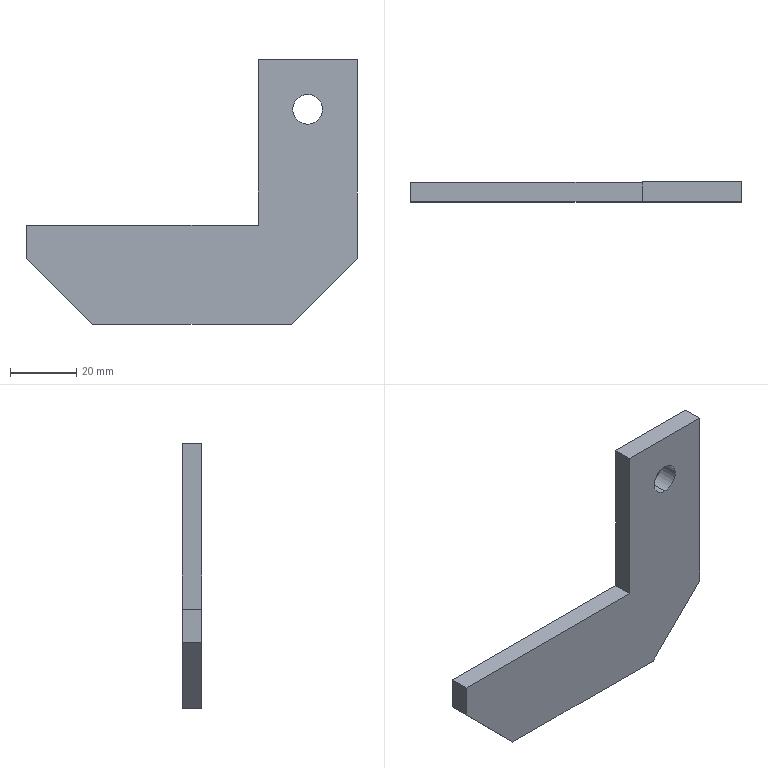Part | SolidWorks | features Chamfer 2, Extrusion 1, ICE 1 | 1 solid | 12 faces | box 100 x 6 x 80 mm | volume 24218 mm3 | plane 10 | cylinder 2 | commonest cylinder face diameters 9 x2
STEP:
#1=CARTESIAN_POINT('',(66.923,0.,-1.423));
#2=VERTEX_POINT('',#1);
#3=CARTESIAN_POINT('',(66.923,0.,7.577));
#4=VERTEX_POINT('',#3);
#5=CARTESIAN_POINT('',(66.923,0.,3.077));
#6=DIRECTION('',(0.,1.,0.));
#7=DIRECTION('',(0.,0.,1.));
#8=AXIS2_PLACEMENT_3D('',#5,#6,#7);
#9=CIRCLE('',#8,4.5);
#10=EDGE_CURVE('',#2,#4,#9,.T.);
#11=ORIENTED_EDGE('',*,*,#10,.F.);
#12=CARTESIAN_POINT('',(66.923,6.,-1.423));
#13=VERTEX_POINT('',#12);
#14=CARTESIAN_POINT('',(66.923,0.,-1.423));
#15=DIRECTION('',(0.,1.,0.));
#16=VECTOR('',#15,1000.);
#17=LINE('',#14,#16);
#18=EDGE_CURVE('',#2,#13,#17,.T.);
#19=ORIENTED_EDGE('',*,*,#18,.T.);
#20=CARTESIAN_POINT('',(66.923,6.,7.577));
#21=VERTEX_POINT('',#20);
#22=CARTESIAN_POINT('',(66.923,6.,3.077));
#23=DIRECTION('',(0.,1.,0.));
#24=DIRECTION('',(0.,0.,1.));
#25=AXIS2_PLACEMENT_3D('',#22,#23,#24);
#26=CIRCLE('',#25,4.5);
#27=EDGE_CURVE('',#13,#21,#26,.T.);
#28=ORIENTED_EDGE('',*,*,#27,.T.);
#29=CARTESIAN_POINT('',(66.923,0.,7.577));
#30=DIRECTION('',(0.,1.,0.));
#31=VECTOR('',#30,1000.);
#32=LINE('',#29,#31);
#33=EDGE_CURVE('',#4,#21,#32,.T.);
#34=ORIENTED_EDGE('',*,*,#33,.F.);
#35=EDGE_LOOP('',(#11,#19,#28,#34));
#36=FACE_OUTER_BOUND('',#35,.T.);
#37=CARTESIAN_POINT('',(66.923,0.,3.077));
#38=DIRECTION('',(0.,1.,0.));
#39=DIRECTION('',(0.,0.,1.));
#40=AXIS2_PLACEMENT_3D('',#37,#38,#39);
#41=CYLINDRICAL_SURFACE('',#40,4.5);
#42=ADVANCED_FACE('',(#36),#41,.F.);
#43=CARTESIAN_POINT('',(-18.077,6.,-41.923));
#44=VERTEX_POINT('',#43);
#45=CARTESIAN_POINT('',(-18.077,6.,-31.923));
#46=VERTEX_POINT('',#45);
#47=CARTESIAN_POINT('',(-18.077,6.,-31.923));
#48=DIRECTION('',(0.,0.,1.));
#49=VECTOR('',#48,1000.);
#50=LINE('',#47,#49);
#51=EDGE_CURVE('',#44,#46,#50,.T.);
#52=ORIENTED_EDGE('',*,*,#51,.F.);
#53=CARTESIAN_POINT('',(-18.077,0.,-41.923));
#54=VERTEX_POINT('',#53);
#55=CARTESIAN_POINT('',(-18.077,6.,-41.923));
#56=DIRECTION('',(0.,-1.,0.));
#57=VECTOR('',#56,1000.);
#58=LINE('',#55,#57);
#59=EDGE_CURVE('',#44,#54,#58,.T.);
#60=ORIENTED_EDGE('',*,*,#59,.T.);
#61=CARTESIAN_POINT('',(-18.077,0.,-31.923));
#62=VERTEX_POINT('',#61);
#63=CARTESIAN_POINT('',(-18.077,0.,-31.923));
#64=DIRECTION('',(0.,0.,1.));
#65=VECTOR('',#64,1000.);
#66=LINE('',#63,#65);
#67=EDGE_CURVE('',#54,#62,#66,.T.);
#68=ORIENTED_EDGE('',*,*,#67,.T.);
#69=CARTESIAN_POINT('',(-18.077,6.,-31.923));
#70=DIRECTION('',(0.,-1.,0.));
#71=VECTOR('',#70,1000.);
#72=LINE('',#69,#71);
#73=EDGE_CURVE('',#46,#62,#72,.T.);
#74=ORIENTED_EDGE('',*,*,#73,.F.);
#75=EDGE_LOOP('',(#52,#60,#68,#74));
#76=FACE_OUTER_BOUND('',#75,.T.);
#77=CARTESIAN_POINT('',(-18.077,6.,-31.923));
#78=DIRECTION('',(1.,0.,0.));
#79=DIRECTION('',(0.,0.,-1.));
#80=AXIS2_PLACEMENT_3D('',#77,#78,#79);
#81=PLANE('',#80);
#82=ADVANCED_FACE('',(#76),#81,.F.);
#83=CARTESIAN_POINT('',(51.923,0.,-31.923));
#84=VERTEX_POINT('',#83);
#85=CARTESIAN_POINT('',(51.923,0.,-31.923));
#86=DIRECTION('',(1.,0.,0.));
#87=VECTOR('',#86,1000.);
#88=LINE('',#85,#87);
#89=EDGE_CURVE('',#62,#84,#88,.T.);
#90=ORIENTED_EDGE('',*,*,#89,.T.);
#91=CARTESIAN_POINT('',(51.923,6.,-31.923));
#92=VERTEX_POINT('',#91);
#93=CARTESIAN_POINT('',(51.923,6.,-31.923));
#94=DIRECTION('',(0.,-1.,0.));
#95=VECTOR('',#94,1000.);
#96=LINE('',#93,#95);
#97=EDGE_CURVE('',#92,#84,#96,.T.);
#98=ORIENTED_EDGE('',*,*,#97,.F.);
#99=CARTESIAN_POINT('',(51.923,6.,-31.923));
#100=DIRECTION('',(1.,0.,0.));
#101=VECTOR('',#100,1000.);
#102=LINE('',#99,#101);
#103=EDGE_CURVE('',#46,#92,#102,.T.);
#104=ORIENTED_EDGE('',*,*,#103,.F.);
#105=ORIENTED_EDGE('',*,*,#73,.T.);
#106=EDGE_LOOP('',(#90,#98,#104,#105));
#107=FACE_OUTER_BOUND('',#106,.T.);
#108=CARTESIAN_POINT('',(51.923,6.,-31.923));
#109=DIRECTION('',(0.,0.,-1.));
#110=DIRECTION('',(-1.,0.,0.));
#111=AXIS2_PLACEMENT_3D('',#108,#109,#110);
#112=PLANE('',#111);
#113=ADVANCED_FACE('',(#107),#112,.F.);
#114=CARTESIAN_POINT('',(51.923,0.,18.077));
#115=VERTEX_POINT('',#114);
#116=CARTESIAN_POINT('',(51.923,0.,18.077));
#117=DIRECTION('',(0.,0.,1.));
#118=VECTOR('',#117,1000.);
#119=LINE('',#116,#118);
#120=EDGE_CURVE('',#84,#115,#119,.T.);
#121=ORIENTED_EDGE('',*,*,#120,.T.);
#122=CARTESIAN_POINT('',(51.923,6.,18.077));
#123=VERTEX_POINT('',#122);
#124=CARTESIAN_POINT('',(51.923,6.,18.077));
#125=DIRECTION('',(0.,-1.,0.));
#126=VECTOR('',#125,1000.);
#127=LINE('',#124,#126);
#128=EDGE_CURVE('',#123,#115,#127,.T.);
#129=ORIENTED_EDGE('',*,*,#128,.F.);
#130=CARTESIAN_POINT('',(51.923,6.,18.077));
#131=DIRECTION('',(0.,0.,1.));
#132=VECTOR('',#131,1000.);
#133=LINE('',#130,#132);
#134=EDGE_CURVE('',#92,#123,#133,.T.);
#135=ORIENTED_EDGE('',*,*,#134,.F.);
#136=ORIENTED_EDGE('',*,*,#97,.T.);
#137=EDGE_LOOP('',(#121,#129,#135,#136));
#138=FACE_OUTER_BOUND('',#137,.T.);
#139=CARTESIAN_POINT('',(51.923,6.,18.077));
#140=DIRECTION('',(1.,0.,0.));
#141=DIRECTION('',(0.,0.,-1.));
#142=AXIS2_PLACEMENT_3D('',#139,#140,#141);
#143=PLANE('',#142);
#144=ADVANCED_FACE('',(#138),#143,.F.);
#145=CARTESIAN_POINT('',(81.923,0.,18.077));
#146=VERTEX_POINT('',#145);
#147=CARTESIAN_POINT('',(81.923,0.,18.077));
#148=DIRECTION('',(1.,0.,0.));
#149=VECTOR('',#148,1000.);
#150=LINE('',#147,#149);
#151=EDGE_CURVE('',#115,#146,#150,.T.);
#152=ORIENTED_EDGE('',*,*,#151,.T.);
#153=CARTESIAN_POINT('',(81.923,6.,18.077));
#154=VERTEX_POINT('',#153);
#155=CARTESIAN_POINT('',(81.923,6.,18.077));
#156=DIRECTION('',(0.,-1.,0.));
#157=VECTOR('',#156,1000.);
#158=LINE('',#155,#157);
#159=EDGE_CURVE('',#154,#146,#158,.T.);
#160=ORIENTED_EDGE('',*,*,#159,.F.);
#161=CARTESIAN_POINT('',(81.923,6.,18.077));
#162=DIRECTION('',(1.,0.,0.));
#163=VECTOR('',#162,1000.);
#164=LINE('',#161,#163);
#165=EDGE_CURVE('',#123,#154,#164,.T.);
#166=ORIENTED_EDGE('',*,*,#165,.F.);
#167=ORIENTED_EDGE('',*,*,#128,.T.);
#168=EDGE_LOOP('',(#152,#160,#166,#167));
#169=FACE_OUTER_BOUND('',#168,.T.);
#170=CARTESIAN_POINT('',(81.923,6.,18.077));
#171=DIRECTION('',(0.,0.,-1.));
#172=DIRECTION('',(-1.,0.,0.));
#173=AXIS2_PLACEMENT_3D('',#170,#171,#172);
#174=PLANE('',#173);
#175=ADVANCED_FACE('',(#169),#174,.F.);
#176=CARTESIAN_POINT('',(81.923,0.,-41.923));
#177=VERTEX_POINT('',#176);
#178=CARTESIAN_POINT('',(81.923,0.,-61.923));
#179=DIRECTION('',(0.,0.,-1.));
#180=VECTOR('',#179,1000.);
#181=LINE('',#178,#180);
#182=EDGE_CURVE('',#146,#177,#181,.T.);
#183=ORIENTED_EDGE('',*,*,#182,.T.);
#184=CARTESIAN_POINT('',(81.923,6.,-41.923));
#185=VERTEX_POINT('',#184);
#186=CARTESIAN_POINT('',(81.923,6.,-41.923));
#187=DIRECTION('',(0.,1.,0.));
#188=VECTOR('',#187,1000.);
#189=LINE('',#186,#188);
#190=EDGE_CURVE('',#177,#185,#189,.T.);
#191=ORIENTED_EDGE('',*,*,#190,.T.);
#192=CARTESIAN_POINT('',(81.923,6.,-61.923));
#193=DIRECTION('',(0.,0.,-1.));
#194=VECTOR('',#193,1000.);
#195=LINE('',#192,#194);
#196=EDGE_CURVE('',#154,#185,#195,.T.);
#197=ORIENTED_EDGE('',*,*,#196,.F.);
#198=ORIENTED_EDGE('',*,*,#159,.T.);
#199=EDGE_LOOP('',(#183,#191,#197,#198));
#200=FACE_OUTER_BOUND('',#199,.T.);
#201=CARTESIAN_POINT('',(81.923,6.,-61.923));
#202=DIRECTION('',(-1.,0.,0.));
#203=DIRECTION('',(0.,0.,1.));
#204=AXIS2_PLACEMENT_3D('',#201,#202,#203);
#205=PLANE('',#204);
#206=ADVANCED_FACE('',(#200),#205,.F.);
#207=CARTESIAN_POINT('',(61.923,6.,-61.923));
#208=VERTEX_POINT('',#207);
#209=CARTESIAN_POINT('',(1.923,6.,-61.923));
#210=VERTEX_POINT('',#209);
#211=CARTESIAN_POINT('',(-18.077,6.,-61.923));
#212=DIRECTION('',(-1.,0.,0.));
#213=VECTOR('',#212,1000.);
#214=LINE('',#211,#213);
#215=EDGE_CURVE('',#208,#210,#214,.T.);
#216=ORIENTED_EDGE('',*,*,#215,.F.);
#217=CARTESIAN_POINT('',(61.923,0.,-61.923));
#218=VERTEX_POINT('',#217);
#219=CARTESIAN_POINT('',(61.923,6.,-61.923));
#220=DIRECTION('',(0.,-1.,0.));
#221=VECTOR('',#220,1000.);
#222=LINE('',#219,#221);
#223=EDGE_CURVE('',#208,#218,#222,.T.);
#224=ORIENTED_EDGE('',*,*,#223,.T.);
#225=CARTESIAN_POINT('',(1.923,0.,-61.923));
#226=VERTEX_POINT('',#225);
#227=CARTESIAN_POINT('',(-18.077,0.,-61.923));
#228=DIRECTION('',(-1.,0.,0.));
#229=VECTOR('',#228,1000.);
#230=LINE('',#227,#229);
#231=EDGE_CURVE('',#218,#226,#230,.T.);
#232=ORIENTED_EDGE('',*,*,#231,.T.);
#233=CARTESIAN_POINT('',(1.923,6.,-61.923));
#234=DIRECTION('',(0.,1.,0.));
#235=VECTOR('',#234,1000.);
#236=LINE('',#233,#235);
#237=EDGE_CURVE('',#226,#210,#236,.T.);
#238=ORIENTED_EDGE('',*,*,#237,.T.);
#239=EDGE_LOOP('',(#216,#224,#232,#238));
#240=FACE_OUTER_BOUND('',#239,.T.);
#241=CARTESIAN_POINT('',(-18.077,6.,-61.923));
#242=DIRECTION('',(0.,0.,1.));
#243=DIRECTION('',(1.,0.,0.));
#244=AXIS2_PLACEMENT_3D('',#241,#242,#243);
#245=PLANE('',#244);
#246=ADVANCED_FACE('',(#240),#245,.F.);
#247=CARTESIAN_POINT('',(66.923,6.,3.077));
#248=DIRECTION('',(0.,1.,0.));
#249=DIRECTION('',(0.,0.,1.));
#250=AXIS2_PLACEMENT_3D('',#247,#248,#249);
#251=CIRCLE('',#250,4.5);
#252=EDGE_CURVE('',#21,#13,#251,.T.);
#253=ORIENTED_EDGE('',*,*,#252,.F.);
#254=ORIENTED_EDGE('',*,*,#27,.F.);
#255=EDGE_LOOP('',(#253,#254));
#256=FACE_BOUND('',#255,.T.);
#257=ORIENTED_EDGE('',*,*,#196,.T.);
#258=CARTESIAN_POINT('',(61.923,6.,-61.923));
#259=DIRECTION('',(-0.7071,0.,-0.7071));
#260=VECTOR('',#259,1000.);
#261=LINE('',#258,#260);
#262=EDGE_CURVE('',#185,#208,#261,.T.);
#263=ORIENTED_EDGE('',*,*,#262,.T.);
#264=ORIENTED_EDGE('',*,*,#215,.T.);
#265=CARTESIAN_POINT('',(-18.077,6.,-41.923));
#266=DIRECTION('',(-0.7071,0.,0.7071));
#267=VECTOR('',#266,1000.);
#268=LINE('',#265,#267);
#269=EDGE_CURVE('',#210,#44,#268,.T.);
#270=ORIENTED_EDGE('',*,*,#269,.T.);
#271=ORIENTED_EDGE('',*,*,#51,.T.);
#272=ORIENTED_EDGE('',*,*,#103,.T.);
#273=ORIENTED_EDGE('',*,*,#134,.T.);
#274=ORIENTED_EDGE('',*,*,#165,.T.);
#275=EDGE_LOOP('',(#257,#263,#264,#270,#271,#272,#273,#274));
#276=FACE_OUTER_BOUND('',#275,.T.);
#277=CARTESIAN_POINT('',(0.,6.,0.));
#278=DIRECTION('',(0.,-1.,0.));
#279=DIRECTION('',(0.,0.,-1.));
#280=AXIS2_PLACEMENT_3D('',#277,#278,#279);
#281=PLANE('',#280);
#282=ADVANCED_FACE('',(#256,#276),#281,.F.);
#283=CARTESIAN_POINT('',(66.923,0.,3.077));
#284=DIRECTION('',(0.,1.,0.));
#285=DIRECTION('',(0.,0.,1.));
#286=AXIS2_PLACEMENT_3D('',#283,#284,#285);
#287=CIRCLE('',#286,4.5);
#288=EDGE_CURVE('',#4,#2,#287,.T.);
#289=ORIENTED_EDGE('',*,*,#288,.T.);
#290=ORIENTED_EDGE('',*,*,#10,.T.);
#291=EDGE_LOOP('',(#289,#290));
#292=FACE_BOUND('',#291,.T.);
#293=ORIENTED_EDGE('',*,*,#231,.F.);
#294=CARTESIAN_POINT('',(61.923,0.,-61.923));
#295=DIRECTION('',(0.7071,0.,0.7071));
#296=VECTOR('',#295,1000.);
#297=LINE('',#294,#296);
#298=EDGE_CURVE('',#218,#177,#297,.T.);
#299=ORIENTED_EDGE('',*,*,#298,.T.);
#300=ORIENTED_EDGE('',*,*,#182,.F.);
#301=ORIENTED_EDGE('',*,*,#151,.F.);
#302=ORIENTED_EDGE('',*,*,#120,.F.);
#303=ORIENTED_EDGE('',*,*,#89,.F.);
#304=ORIENTED_EDGE('',*,*,#67,.F.);
#305=CARTESIAN_POINT('',(-30.,0.,-30.));
#306=DIRECTION('',(0.7071,0.,-0.7071));
#307=VECTOR('',#306,1000.);
#308=LINE('',#305,#307);
#309=EDGE_CURVE('',#54,#226,#308,.T.);
#310=ORIENTED_EDGE('',*,*,#309,.T.);
#311=EDGE_LOOP('',(#293,#299,#300,#301,#302,#303,#304,#310));
#312=FACE_OUTER_BOUND('',#311,.T.);
#313=CARTESIAN_POINT('',(0.,0.,0.));
#314=DIRECTION('',(0.,-1.,0.));
#315=DIRECTION('',(0.,0.,-1.));
#316=AXIS2_PLACEMENT_3D('',#313,#314,#315);
#317=PLANE('',#316);
#318=ADVANCED_FACE('',(#292,#312),#317,.T.);
#319=ORIENTED_EDGE('',*,*,#18,.F.);
#320=ORIENTED_EDGE('',*,*,#288,.F.);
#321=ORIENTED_EDGE('',*,*,#33,.T.);
#322=ORIENTED_EDGE('',*,*,#252,.T.);
#323=EDGE_LOOP('',(#319,#320,#321,#322));
#324=FACE_OUTER_BOUND('',#323,.T.);
#325=CARTESIAN_POINT('',(66.923,0.,3.077));
#326=DIRECTION('',(0.,1.,0.));
#327=DIRECTION('',(0.,0.,1.));
#328=AXIS2_PLACEMENT_3D('',#325,#326,#327);
#329=CYLINDRICAL_SURFACE('',#328,4.5);
#330=ADVANCED_FACE('',(#324),#329,.F.);
#331=ORIENTED_EDGE('',*,*,#269,.F.);
#332=ORIENTED_EDGE('',*,*,#237,.F.);
#333=ORIENTED_EDGE('',*,*,#309,.F.);
#334=ORIENTED_EDGE('',*,*,#59,.F.);
#335=EDGE_LOOP('',(#331,#332,#333,#334));
#336=FACE_OUTER_BOUND('',#335,.T.);
#337=CARTESIAN_POINT('',(-18.077,6.,-41.923));
#338=DIRECTION('',(0.7071,0.,0.7071));
#339=DIRECTION('',(0.,-1.,0.));
#340=AXIS2_PLACEMENT_3D('',#337,#338,#339);
#341=PLANE('',#340);
#342=ADVANCED_FACE('',(#336),#341,.F.);
#343=ORIENTED_EDGE('',*,*,#262,.F.);
#344=ORIENTED_EDGE('',*,*,#190,.F.);
#345=ORIENTED_EDGE('',*,*,#298,.F.);
#346=ORIENTED_EDGE('',*,*,#223,.F.);
#347=EDGE_LOOP('',(#343,#344,#345,#346));
#348=FACE_OUTER_BOUND('',#347,.T.);
#349=CARTESIAN_POINT('',(61.923,6.,-61.923));
#350=DIRECTION('',(-0.7071,0.,0.7071));
#351=DIRECTION('',(0.,-1.,0.));
#352=AXIS2_PLACEMENT_3D('',#349,#350,#351);
#353=PLANE('',#352);
#354=ADVANCED_FACE('',(#348),#353,.F.);
#355=CLOSED_SHELL('',(#42,#82,#113,#144,#175,#206,#246,#282,#318,#330,#342,#354));
#356=MANIFOLD_SOLID_BREP('',#355);
#357=CARTESIAN_POINT('',(0.,0.,0.));
#358=DIRECTION('',(0.,0.,1.));
#359=DIRECTION('',(1.,0.,0.));
#360=AXIS2_PLACEMENT_3D('',#357,#358,#359);
#361=(LENGTH_UNIT()NAMED_UNIT(*)SI_UNIT(.MILLI.,.METRE.));
#362=UNCERTAINTY_MEASURE_WITH_UNIT(LENGTH_MEASURE(0.00001),#361,'','');
#363=(NAMED_UNIT(*)PLANE_ANGLE_UNIT()SI_UNIT($,.RADIAN.));
#364=(NAMED_UNIT(*)SI_UNIT($,.STERADIAN.)SOLID_ANGLE_UNIT());
#365=(GEOMETRIC_REPRESENTATION_CONTEXT(3)GLOBAL_UNCERTAINTY_ASSIGNED_CONTEXT((#362))GLOBAL_UNIT_ASSIGNED_CONTEXT((#361,#363,#364))REPRESENTATION_CONTEXT('',''));
#366=ADVANCED_BREP_SHAPE_REPRESENTATION('',(#356,#360),#365);